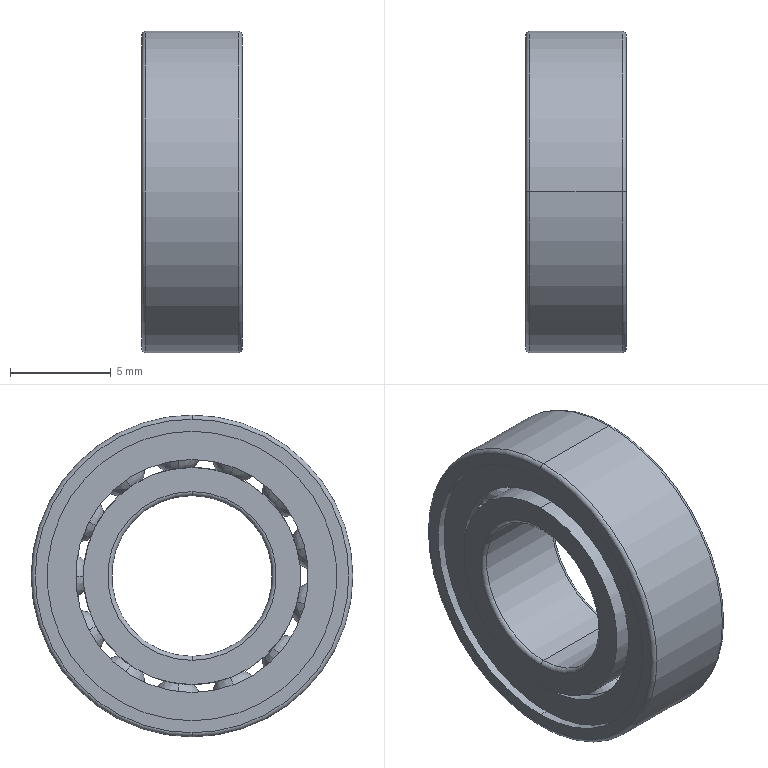Part | SolidWorks | features BaseBody 1 | 1 solid | 264 faces | box 5 x 16 x 16 mm | volume 538.645 mm3 | sphere 156 | torus 50 | plane 34 | cylinder 24 | commonest cylinder face diameters 14.4 x8 10.8 x4 11.592 x4 8 x2 11.94 x2 13.26 x2